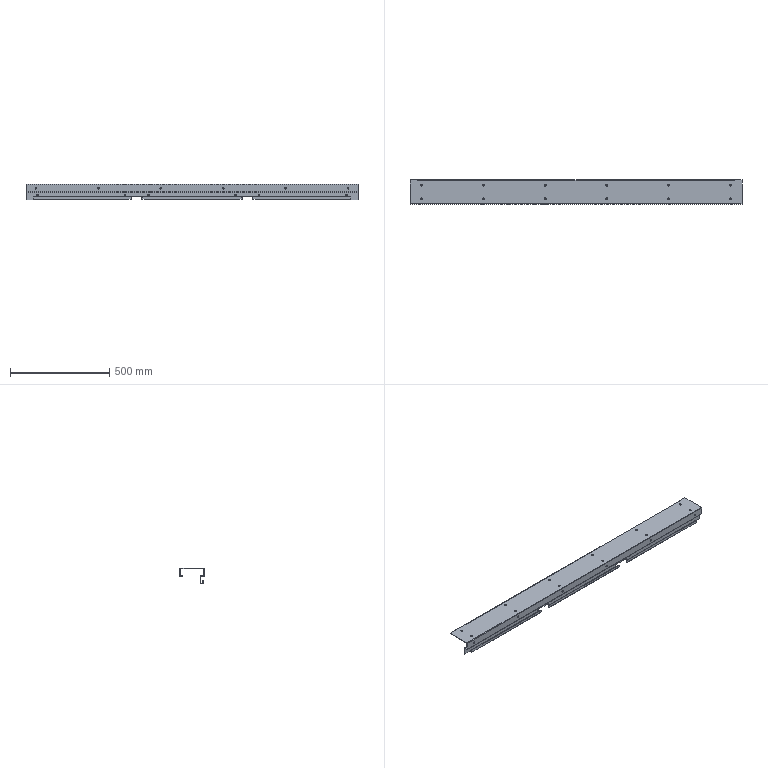Part | STEP file | TS-006-01 | 1 solid | 198 faces | box 1670 x 122 x 78 mm | volume 940094 mm3 | plane 108 | cylinder 90 | commonest cylinder face diameters 8 x24 10 x24 0.4 x13 4.4 x13 5.4 x12 20 x4